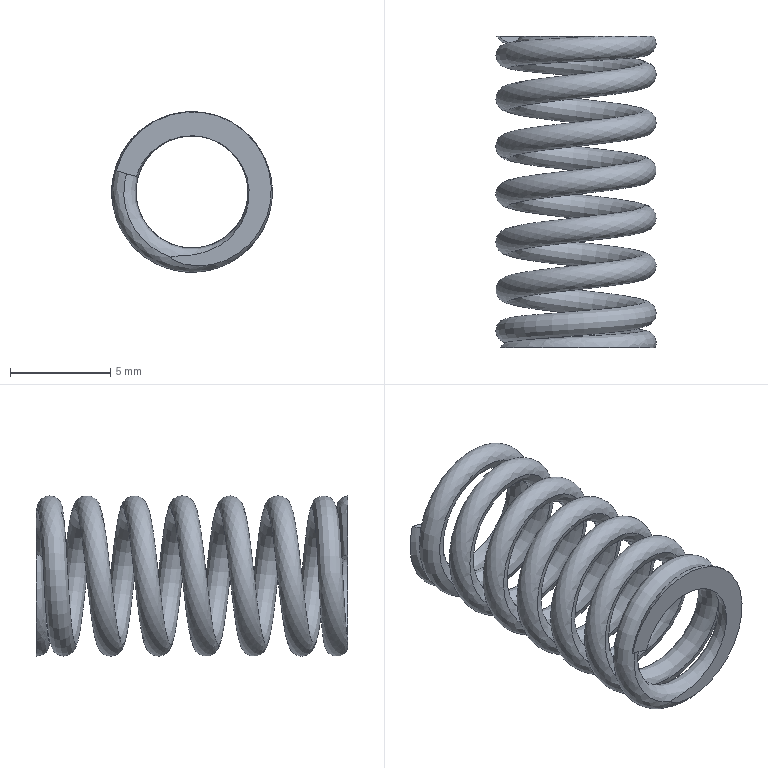Part | SolidWorks | features BaseBody 1 | 1 solid | 6 faces | box 8.001 x 15.5 x 8 mm | volume 180.594 mm3 | plane 4 | spline 2